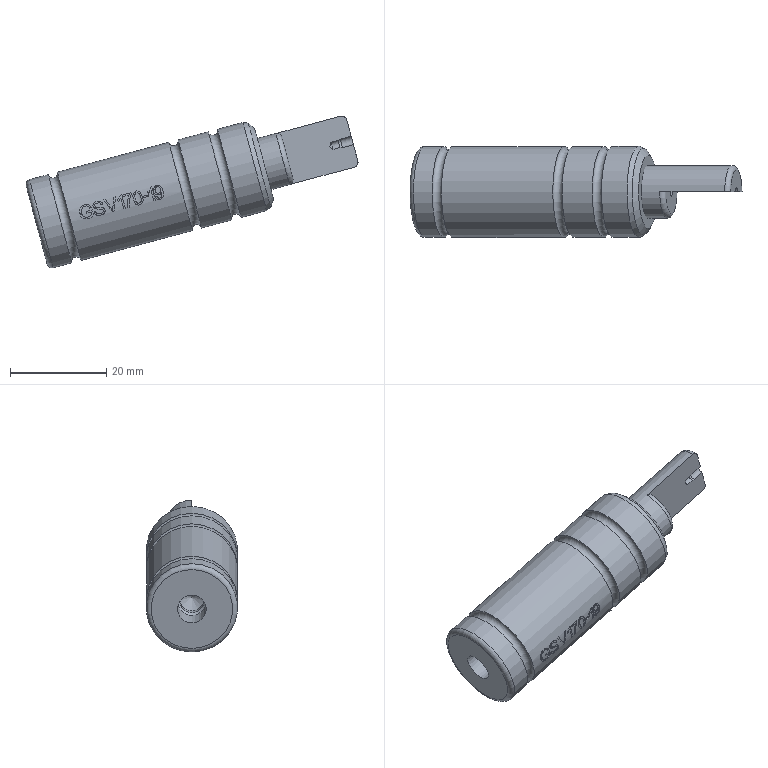Part | NX | features GSV170-19_1 2 | 1 solid | 145 faces | box 69.116 x 19 x 31.639 mm | volume 14434 mm3 | plane 70 | cylinder 61 | cone 8 | torus 6 | commonest cylinder face diameters 18.8 x9 19 x6 1.558 x2 1.833 x2 3.618 x2 4.063 x2